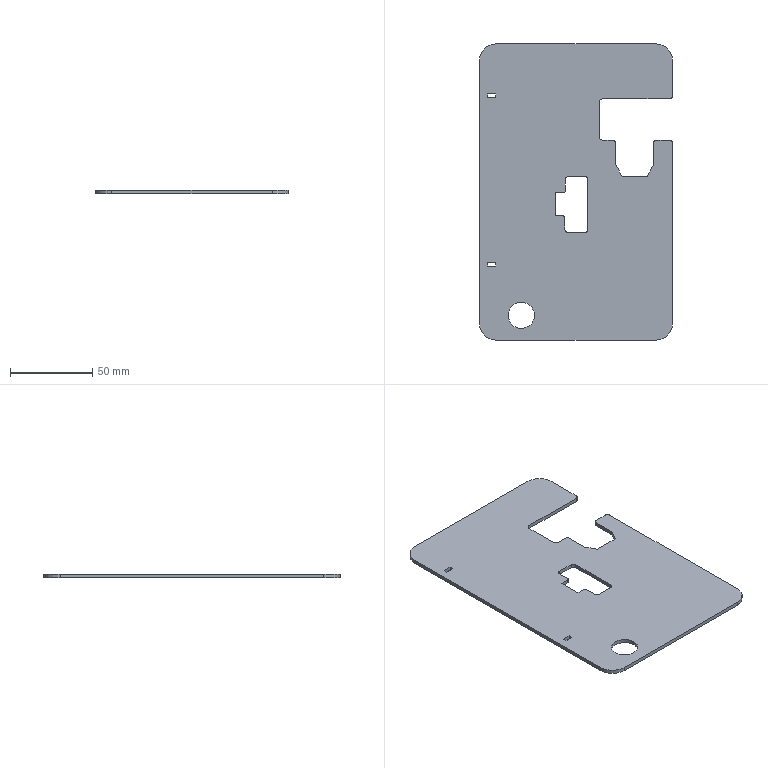Part | SolidWorks | features FlatPattern 1, SMBaseFlange 1, SheetMetal 1 | 1 solid | 50 faces | box 117.378 x 180 x 2.3 mm | volume 42940 mm3 | plane 32 | cylinder 18 | commonest cylinder face diameters 4 x10 20 x4 2 x2 16 x2